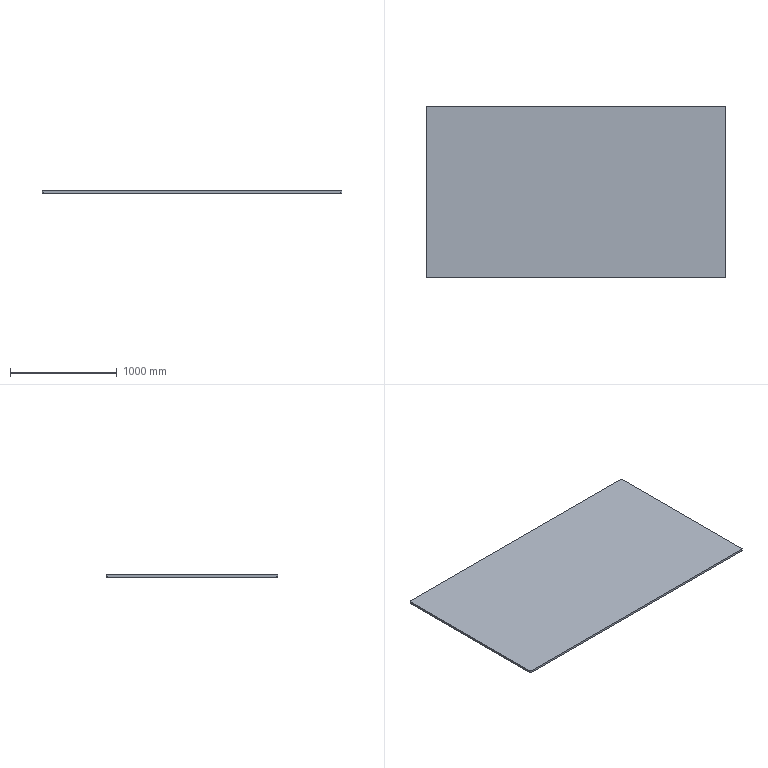Part | STEP file | Part 1 | 1 solid | 10 faces | box 2800 x 1600 x 20 mm | volume 89598283 mm3 | plane 6 | cylinder 4 | commonest cylinder face diameters 20 x4
STEP:
#1=CARTESIAN_POINT('',(1400.,-790.,0.));
#2=VERTEX_POINT('',#1);
#3=CARTESIAN_POINT('',(1400.,790.,0.));
#4=VERTEX_POINT('',#3);
#5=CARTESIAN_POINT('',(1400.,800.,0.));
#6=DIRECTION('',(0.,1.,0.));
#7=VECTOR('',#6,1000.);
#8=LINE('',#5,#7);
#9=EDGE_CURVE('',#2,#4,#8,.T.);
#10=ORIENTED_EDGE('',*,*,#9,.T.);
#11=CARTESIAN_POINT('',(1400.,790.,20.));
#12=VERTEX_POINT('',#11);
#13=CARTESIAN_POINT('',(1400.,790.,20.));
#14=DIRECTION('',(0.,0.,1.));
#15=VECTOR('',#14,1000.);
#16=LINE('',#13,#15);
#17=EDGE_CURVE('',#4,#12,#16,.T.);
#18=ORIENTED_EDGE('',*,*,#17,.T.);
#19=CARTESIAN_POINT('',(1400.,-790.,20.));
#20=VERTEX_POINT('',#19);
#21=CARTESIAN_POINT('',(1400.,800.,20.));
#22=DIRECTION('',(0.,1.,0.));
#23=VECTOR('',#22,1000.);
#24=LINE('',#21,#23);
#25=EDGE_CURVE('',#20,#12,#24,.T.);
#26=ORIENTED_EDGE('',*,*,#25,.F.);
#27=CARTESIAN_POINT('',(1400.,-790.,20.));
#28=DIRECTION('',(0.,0.,-1.));
#29=VECTOR('',#28,1000.);
#30=LINE('',#27,#29);
#31=EDGE_CURVE('',#20,#2,#30,.T.);
#32=ORIENTED_EDGE('',*,*,#31,.T.);
#33=EDGE_LOOP('',(#10,#18,#26,#32));
#34=FACE_OUTER_BOUND('',#33,.T.);
#35=CARTESIAN_POINT('',(1400.,800.,20.));
#36=DIRECTION('',(-1.,0.,0.));
#37=DIRECTION('',(0.,-1.,0.));
#38=AXIS2_PLACEMENT_3D('',#35,#36,#37);
#39=PLANE('',#38);
#40=ADVANCED_FACE('',(#34),#39,.F.);
#41=CARTESIAN_POINT('',(1390.,800.,20.));
#42=VERTEX_POINT('',#41);
#43=CARTESIAN_POINT('',(-1390.,800.,20.));
#44=VERTEX_POINT('',#43);
#45=CARTESIAN_POINT('',(-1400.,800.,20.));
#46=DIRECTION('',(-1.,0.,0.));
#47=VECTOR('',#46,1000.);
#48=LINE('',#45,#47);
#49=EDGE_CURVE('',#42,#44,#48,.T.);
#50=ORIENTED_EDGE('',*,*,#49,.F.);
#51=CARTESIAN_POINT('',(1390.,800.,0.));
#52=VERTEX_POINT('',#51);
#53=CARTESIAN_POINT('',(1390.,800.,20.));
#54=DIRECTION('',(0.,0.,-1.));
#55=VECTOR('',#54,1000.);
#56=LINE('',#53,#55);
#57=EDGE_CURVE('',#42,#52,#56,.T.);
#58=ORIENTED_EDGE('',*,*,#57,.T.);
#59=CARTESIAN_POINT('',(-1390.,800.,0.));
#60=VERTEX_POINT('',#59);
#61=CARTESIAN_POINT('',(-1400.,800.,0.));
#62=DIRECTION('',(-1.,0.,0.));
#63=VECTOR('',#62,1000.);
#64=LINE('',#61,#63);
#65=EDGE_CURVE('',#52,#60,#64,.T.);
#66=ORIENTED_EDGE('',*,*,#65,.T.);
#67=CARTESIAN_POINT('',(-1390.,800.,20.));
#68=DIRECTION('',(0.,0.,1.));
#69=VECTOR('',#68,1000.);
#70=LINE('',#67,#69);
#71=EDGE_CURVE('',#60,#44,#70,.T.);
#72=ORIENTED_EDGE('',*,*,#71,.T.);
#73=EDGE_LOOP('',(#50,#58,#66,#72));
#74=FACE_OUTER_BOUND('',#73,.T.);
#75=CARTESIAN_POINT('',(-1400.,800.,20.));
#76=DIRECTION('',(0.,-1.,0.));
#77=DIRECTION('',(1.,0.,0.));
#78=AXIS2_PLACEMENT_3D('',#75,#76,#77);
#79=PLANE('',#78);
#80=ADVANCED_FACE('',(#74),#79,.F.);
#81=CARTESIAN_POINT('',(-1400.,790.,0.));
#82=VERTEX_POINT('',#81);
#83=CARTESIAN_POINT('',(-1400.,-790.,0.));
#84=VERTEX_POINT('',#83);
#85=CARTESIAN_POINT('',(-1400.,800.,0.));
#86=DIRECTION('',(0.,-1.,0.));
#87=VECTOR('',#86,1000.);
#88=LINE('',#85,#87);
#89=EDGE_CURVE('',#82,#84,#88,.T.);
#90=ORIENTED_EDGE('',*,*,#89,.T.);
#91=CARTESIAN_POINT('',(-1400.,-790.,20.));
#92=VERTEX_POINT('',#91);
#93=CARTESIAN_POINT('',(-1400.,-790.,20.));
#94=DIRECTION('',(0.,0.,1.));
#95=VECTOR('',#94,1000.);
#96=LINE('',#93,#95);
#97=EDGE_CURVE('',#84,#92,#96,.T.);
#98=ORIENTED_EDGE('',*,*,#97,.T.);
#99=CARTESIAN_POINT('',(-1400.,790.,20.));
#100=VERTEX_POINT('',#99);
#101=CARTESIAN_POINT('',(-1400.,800.,20.));
#102=DIRECTION('',(0.,-1.,0.));
#103=VECTOR('',#102,1000.);
#104=LINE('',#101,#103);
#105=EDGE_CURVE('',#100,#92,#104,.T.);
#106=ORIENTED_EDGE('',*,*,#105,.F.);
#107=CARTESIAN_POINT('',(-1400.,790.,20.));
#108=DIRECTION('',(0.,0.,-1.));
#109=VECTOR('',#108,1000.);
#110=LINE('',#107,#109);
#111=EDGE_CURVE('',#100,#82,#110,.T.);
#112=ORIENTED_EDGE('',*,*,#111,.T.);
#113=EDGE_LOOP('',(#90,#98,#106,#112));
#114=FACE_OUTER_BOUND('',#113,.T.);
#115=CARTESIAN_POINT('',(-1400.,800.,20.));
#116=DIRECTION('',(1.,0.,0.));
#117=DIRECTION('',(0.,1.,0.));
#118=AXIS2_PLACEMENT_3D('',#115,#116,#117);
#119=PLANE('',#118);
#120=ADVANCED_FACE('',(#114),#119,.F.);
#121=CARTESIAN_POINT('',(-1390.,-800.,0.));
#122=VERTEX_POINT('',#121);
#123=CARTESIAN_POINT('',(1390.,-800.,0.));
#124=VERTEX_POINT('',#123);
#125=CARTESIAN_POINT('',(-1400.,-800.,0.));
#126=DIRECTION('',(1.,0.,0.));
#127=VECTOR('',#126,1000.);
#128=LINE('',#125,#127);
#129=EDGE_CURVE('',#122,#124,#128,.T.);
#130=ORIENTED_EDGE('',*,*,#129,.T.);
#131=CARTESIAN_POINT('',(1390.,-800.,20.));
#132=VERTEX_POINT('',#131);
#133=CARTESIAN_POINT('',(1390.,-800.,20.));
#134=DIRECTION('',(0.,0.,1.));
#135=VECTOR('',#134,1000.);
#136=LINE('',#133,#135);
#137=EDGE_CURVE('',#124,#132,#136,.T.);
#138=ORIENTED_EDGE('',*,*,#137,.T.);
#139=CARTESIAN_POINT('',(-1390.,-800.,20.));
#140=VERTEX_POINT('',#139);
#141=CARTESIAN_POINT('',(-1400.,-800.,20.));
#142=DIRECTION('',(1.,0.,0.));
#143=VECTOR('',#142,1000.);
#144=LINE('',#141,#143);
#145=EDGE_CURVE('',#140,#132,#144,.T.);
#146=ORIENTED_EDGE('',*,*,#145,.F.);
#147=CARTESIAN_POINT('',(-1390.,-800.,20.));
#148=DIRECTION('',(0.,0.,-1.));
#149=VECTOR('',#148,1000.);
#150=LINE('',#147,#149);
#151=EDGE_CURVE('',#140,#122,#150,.T.);
#152=ORIENTED_EDGE('',*,*,#151,.T.);
#153=EDGE_LOOP('',(#130,#138,#146,#152));
#154=FACE_OUTER_BOUND('',#153,.T.);
#155=CARTESIAN_POINT('',(-1400.,-800.,20.));
#156=DIRECTION('',(0.,1.,0.));
#157=DIRECTION('',(0.,0.,1.));
#158=AXIS2_PLACEMENT_3D('',#155,#156,#157);
#159=PLANE('',#158);
#160=ADVANCED_FACE('',(#154),#159,.F.);
#161=ORIENTED_EDGE('',*,*,#25,.T.);
#162=CARTESIAN_POINT('',(1390.,790.,20.));
#163=DIRECTION('',(0.,0.,1.));
#164=DIRECTION('',(1.,0.,0.));
#165=AXIS2_PLACEMENT_3D('',#162,#163,#164);
#166=CIRCLE('',#165,10.);
#167=EDGE_CURVE('',#12,#42,#166,.T.);
#168=ORIENTED_EDGE('',*,*,#167,.T.);
#169=ORIENTED_EDGE('',*,*,#49,.T.);
#170=CARTESIAN_POINT('',(-1390.,790.,20.));
#171=DIRECTION('',(0.,0.,1.));
#172=DIRECTION('',(1.,0.,0.));
#173=AXIS2_PLACEMENT_3D('',#170,#171,#172);
#174=CIRCLE('',#173,10.);
#175=EDGE_CURVE('',#44,#100,#174,.T.);
#176=ORIENTED_EDGE('',*,*,#175,.T.);
#177=ORIENTED_EDGE('',*,*,#105,.T.);
#178=CARTESIAN_POINT('',(-1390.,-790.,20.));
#179=DIRECTION('',(0.,0.,1.));
#180=DIRECTION('',(1.,0.,0.));
#181=AXIS2_PLACEMENT_3D('',#178,#179,#180);
#182=CIRCLE('',#181,10.);
#183=EDGE_CURVE('',#92,#140,#182,.T.);
#184=ORIENTED_EDGE('',*,*,#183,.T.);
#185=ORIENTED_EDGE('',*,*,#145,.T.);
#186=CARTESIAN_POINT('',(1390.,-790.,20.));
#187=DIRECTION('',(0.,0.,1.));
#188=DIRECTION('',(1.,0.,0.));
#189=AXIS2_PLACEMENT_3D('',#186,#187,#188);
#190=CIRCLE('',#189,10.);
#191=EDGE_CURVE('',#132,#20,#190,.T.);
#192=ORIENTED_EDGE('',*,*,#191,.T.);
#193=EDGE_LOOP('',(#161,#168,#169,#176,#177,#184,#185,#192));
#194=FACE_OUTER_BOUND('',#193,.T.);
#195=CARTESIAN_POINT('',(0.,0.,20.));
#196=DIRECTION('',(0.,0.,1.));
#197=DIRECTION('',(1.,0.,0.));
#198=AXIS2_PLACEMENT_3D('',#195,#196,#197);
#199=PLANE('',#198);
#200=ADVANCED_FACE('',(#194),#199,.T.);
#201=ORIENTED_EDGE('',*,*,#65,.F.);
#202=CARTESIAN_POINT('',(1390.,790.,0.));
#203=DIRECTION('',(0.,0.,-1.));
#204=DIRECTION('',(1.,0.,0.));
#205=AXIS2_PLACEMENT_3D('',#202,#203,#204);
#206=CIRCLE('',#205,10.);
#207=EDGE_CURVE('',#52,#4,#206,.T.);
#208=ORIENTED_EDGE('',*,*,#207,.T.);
#209=ORIENTED_EDGE('',*,*,#9,.F.);
#210=CARTESIAN_POINT('',(1390.,-790.,0.));
#211=DIRECTION('',(0.,0.,-1.));
#212=DIRECTION('',(1.,0.,0.));
#213=AXIS2_PLACEMENT_3D('',#210,#211,#212);
#214=CIRCLE('',#213,10.);
#215=EDGE_CURVE('',#2,#124,#214,.T.);
#216=ORIENTED_EDGE('',*,*,#215,.T.);
#217=ORIENTED_EDGE('',*,*,#129,.F.);
#218=CARTESIAN_POINT('',(-1390.,-790.,0.));
#219=DIRECTION('',(0.,0.,-1.));
#220=DIRECTION('',(1.,0.,0.));
#221=AXIS2_PLACEMENT_3D('',#218,#219,#220);
#222=CIRCLE('',#221,10.);
#223=EDGE_CURVE('',#122,#84,#222,.T.);
#224=ORIENTED_EDGE('',*,*,#223,.T.);
#225=ORIENTED_EDGE('',*,*,#89,.F.);
#226=CARTESIAN_POINT('',(-1390.,790.,0.));
#227=DIRECTION('',(0.,0.,-1.));
#228=DIRECTION('',(1.,0.,0.));
#229=AXIS2_PLACEMENT_3D('',#226,#227,#228);
#230=CIRCLE('',#229,10.);
#231=EDGE_CURVE('',#82,#60,#230,.T.);
#232=ORIENTED_EDGE('',*,*,#231,.T.);
#233=EDGE_LOOP('',(#201,#208,#209,#216,#217,#224,#225,#232));
#234=FACE_OUTER_BOUND('',#233,.T.);
#235=CARTESIAN_POINT('',(0.,0.,0.));
#236=DIRECTION('',(0.,0.,1.));
#237=DIRECTION('',(1.,0.,0.));
#238=AXIS2_PLACEMENT_3D('',#235,#236,#237);
#239=PLANE('',#238);
#240=ADVANCED_FACE('',(#234),#239,.F.);
#241=ORIENTED_EDGE('',*,*,#167,.F.);
#242=ORIENTED_EDGE('',*,*,#17,.F.);
#243=ORIENTED_EDGE('',*,*,#207,.F.);
#244=ORIENTED_EDGE('',*,*,#57,.F.);
#245=EDGE_LOOP('',(#241,#242,#243,#244));
#246=FACE_OUTER_BOUND('',#245,.T.);
#247=CARTESIAN_POINT('',(1390.,790.,20.));
#248=DIRECTION('',(0.,0.,-1.));
#249=DIRECTION('',(-1.,0.,0.));
#250=AXIS2_PLACEMENT_3D('',#247,#248,#249);
#251=CYLINDRICAL_SURFACE('',#250,10.);
#252=ADVANCED_FACE('',(#246),#251,.T.);
#253=ORIENTED_EDGE('',*,*,#191,.F.);
#254=ORIENTED_EDGE('',*,*,#137,.F.);
#255=ORIENTED_EDGE('',*,*,#215,.F.);
#256=ORIENTED_EDGE('',*,*,#31,.F.);
#257=EDGE_LOOP('',(#253,#254,#255,#256));
#258=FACE_OUTER_BOUND('',#257,.T.);
#259=CARTESIAN_POINT('',(1390.,-790.,20.));
#260=DIRECTION('',(0.,0.,-1.));
#261=DIRECTION('',(-1.,0.,0.));
#262=AXIS2_PLACEMENT_3D('',#259,#260,#261);
#263=CYLINDRICAL_SURFACE('',#262,10.);
#264=ADVANCED_FACE('',(#258),#263,.T.);
#265=ORIENTED_EDGE('',*,*,#183,.F.);
#266=ORIENTED_EDGE('',*,*,#97,.F.);
#267=ORIENTED_EDGE('',*,*,#223,.F.);
#268=ORIENTED_EDGE('',*,*,#151,.F.);
#269=EDGE_LOOP('',(#265,#266,#267,#268));
#270=FACE_OUTER_BOUND('',#269,.T.);
#271=CARTESIAN_POINT('',(-1390.,-790.,20.));
#272=DIRECTION('',(0.,0.,-1.));
#273=DIRECTION('',(-1.,0.,0.));
#274=AXIS2_PLACEMENT_3D('',#271,#272,#273);
#275=CYLINDRICAL_SURFACE('',#274,10.);
#276=ADVANCED_FACE('',(#270),#275,.T.);
#277=ORIENTED_EDGE('',*,*,#175,.F.);
#278=ORIENTED_EDGE('',*,*,#71,.F.);
#279=ORIENTED_EDGE('',*,*,#231,.F.);
#280=ORIENTED_EDGE('',*,*,#111,.F.);
#281=EDGE_LOOP('',(#277,#278,#279,#280));
#282=FACE_OUTER_BOUND('',#281,.T.);
#283=CARTESIAN_POINT('',(-1390.,790.,20.));
#284=DIRECTION('',(0.,0.,-1.));
#285=DIRECTION('',(-1.,0.,0.));
#286=AXIS2_PLACEMENT_3D('',#283,#284,#285);
#287=CYLINDRICAL_SURFACE('',#286,10.);
#288=ADVANCED_FACE('',(#282),#287,.T.);
#289=CLOSED_SHELL('',(#40,#80,#120,#160,#200,#240,#252,#264,#276,#288));
#290=MANIFOLD_SOLID_BREP('',#289);
#291=CARTESIAN_POINT('',(0.,0.,0.));
#292=DIRECTION('',(0.,0.,1.));
#293=DIRECTION('',(1.,0.,0.));
#294=AXIS2_PLACEMENT_3D('',#291,#292,#293);
#295=(LENGTH_UNIT()NAMED_UNIT(*)SI_UNIT(.MILLI.,.METRE.));
#296=UNCERTAINTY_MEASURE_WITH_UNIT(LENGTH_MEASURE(0.00001),#295,'','');
#297=(NAMED_UNIT(*)PLANE_ANGLE_UNIT()SI_UNIT($,.RADIAN.));
#298=(NAMED_UNIT(*)SI_UNIT($,.STERADIAN.)SOLID_ANGLE_UNIT());
#299=(GEOMETRIC_REPRESENTATION_CONTEXT(3)GLOBAL_UNCERTAINTY_ASSIGNED_CONTEXT((#296))GLOBAL_UNIT_ASSIGNED_CONTEXT((#295,#297,#298))REPRESENTATION_CONTEXT('',''));
#300=ADVANCED_BREP_SHAPE_REPRESENTATION('',(#290,#294),#299);